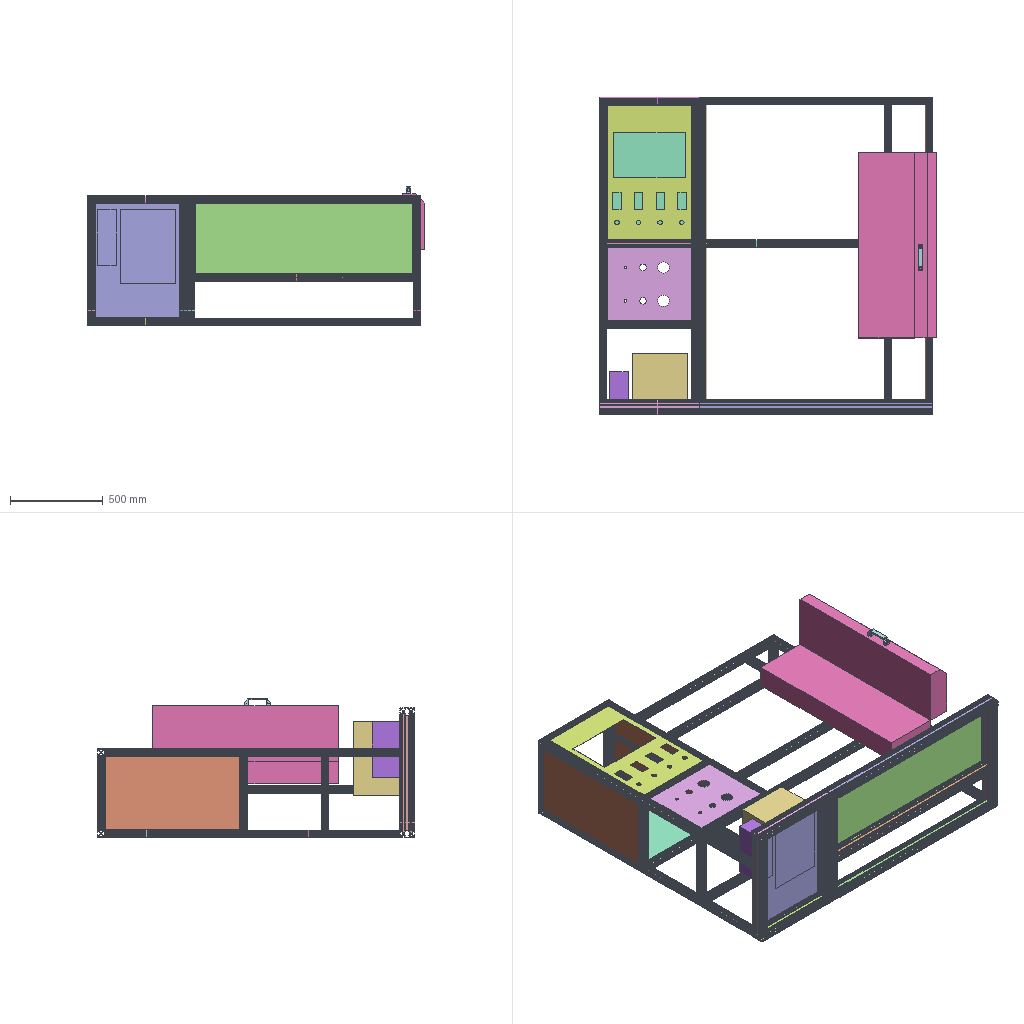Assembly | SolidWorks | 17 different items | 19 placed | box 1821 x 1715 x 750 mm
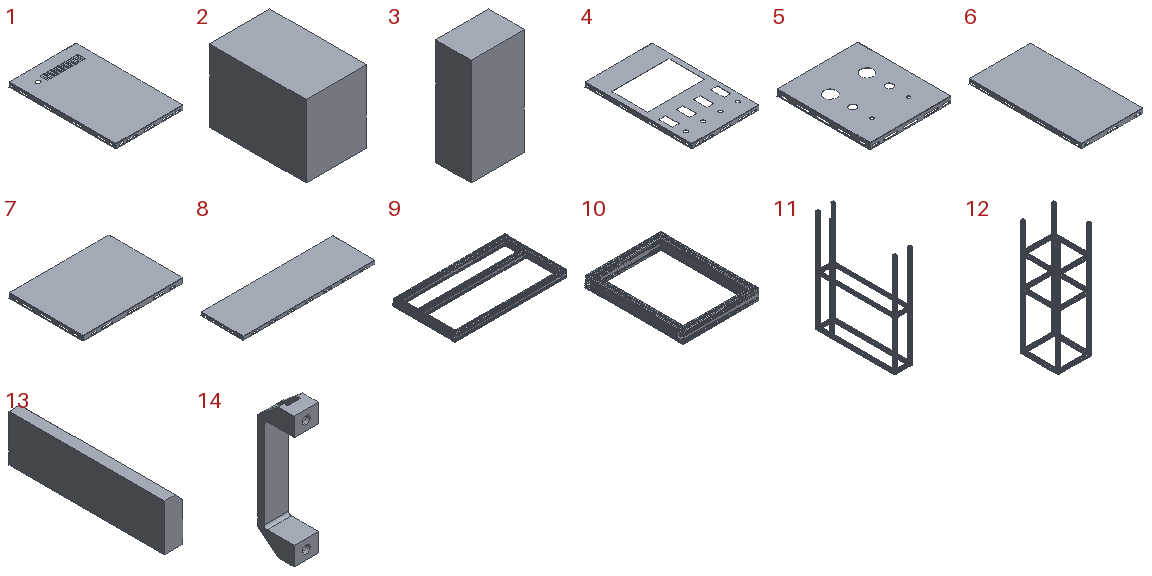Parts list (item | name | quantity | size | volume | features):
1 | - | x1 | 459 x 729 x 30 mm | 574629 mm3 | features ICE 3, EdgeFlange 1, FlatPattern 1, SMBaseFlange 1, SheetMetal 1
2 | - | x1 | 250 x 400 x 300 mm | 30000000 mm3 | features Extrusion 1
3 | - | x1 | 150 x 100 x 300 mm | 4500000 mm3 | features Extrusion 1
4 | - | x1 | 459 x 729 x 30 mm | 412274 mm3 | features ICE 3, EdgeFlange 1, FlatPattern 1, SMBaseFlange 1, SheetMetal 1
5 | - | x1 | 399 x 459 x 30 mm | 317293 mm3 | features ICE 2, Cut 1, EdgeFlange 1, FlatPattern 1, SMBaseFlange 1, SheetMetal 1
6 | - | x2 | 399 x 729 x 30 mm | 516047 mm3 | features ICE 2, EdgeFlange 1, FlatPattern 1, SMBaseFlange 1, SheetMetal 1
7 | - | x1 | 619 x 459 x 30 mm | 499692 mm3 | features ICE 2, EdgeFlange 1, FlatPattern 1, SMBaseFlange 1, SheetMetal 1
8 | - | x1 | 1179 x 379 x 30 mm | 777868 mm3 | features ICE 2, EdgeFlange 1, FlatPattern 1, SMBaseFlange 1, SheetMetal 1
9 | - | x1 | 1260 x 700.002 x 80 mm | 4888550 mm3 | features 3DProfileFeature 1, ICE 1, WeldCornerFeat 1, WeldMemberFeat 1, WeldmentFeature 1
10 | - | x1 | 540.002 x 700.002 x 80 mm | 2304321 mm3 | features 3DProfileFeature 1, ICE 1, WeldCornerFeat 1, WeldMemberFeat 1, WeldmentFeature 1
11 | - | x1 | 280 x 1260 x 1635 mm | 6460308 mm3 | features WeldCornerFeat 18, WeldMemberFeat 9, 3DProfileFeature 2, ICE 1, WeldmentFeature 1
12 | - | x1 | 480 x 540 x 1635 mm | 5554976 mm3 | features WeldCornerFeat 16, WeldMemberFeat 8, 3DProfileFeature 1, ICE 1, WeldmentFeature 1
13 | - | x2 | 120 x 1000 x 300 mm | 34750000 mm3 | features Chamfer 1, Extrusion 1
14 | - | x1 | 26 x 39 x 140 mm | 37768 mm3 | features BaseBody 1
15 | E-DEPN-W1-80-N(JLC FA) | x1 | - | - | -
16 | Base Plate2 | x1 | - | - | -
17 | Base Plate5 | x1 | - | - | -
Mates (type | each side: item.copy, entity, surface, feature):
Coincident | 10.1 plane | assembly plane | 3 times
Coincident | 12.1 face plane Aluminum Profile 40 X 40L X R4.5(6) | 4.1 face plane Base-Flange1
Width | 4.1 face plane Edge-Flange1 | 4.1 face plane Edge-Flange1 | 12.1 face plane Aluminum Profile 40 X 40L X R4.5(1) | 12.1 face plane Aluminum Profile 40 X 40L X R4.5(1)
Width | 4.1 face plane Edge-Flange1 | 4.1 face plane Edge-Flange1 | 12.1 face plane Aluminum Profile 40 X 40L X R4.5(6) | 12.1 face plane Aluminum Profile 40 X 40L X R4.5(2)
Width | 6.1 face plane Edge-Flange1 | 6.1 face plane Edge-Flange1 | 12.1 face plane Aluminum Profile 40 X 40L X R4.5(1) | 12.1 face plane Aluminum Profile 40 X 40L X R4.5(1)
Width | 6.1 face plane Edge-Flange1 | 6.1 face plane Edge-Flange1 | 12.1 face plane Aluminum Profile 40 X 40L X R4.5(2) | 12.1 face plane Aluminum Profile 40 X 40L X R4.5(10)
Coincident | 12.1 face plane Aluminum Profile 40 X 40L X R4.5(10) | 6.1 face plane Base-Flange1
Width | 1.1 face plane Edge-Flange1 | 1.1 face plane Edge-Flange1 | 12.1 face plane Aluminum Profile 40 X 40L X R4.5(6) | 12.1 face plane Aluminum Profile 40 X 40L X R4.5(2)
Width | 1.1 face plane Edge-Flange1 | 1.1 face plane Edge-Flange1 | 12.1 face plane Aluminum Profile 40 X 40L X R4.5(1) | 12.1 face plane Aluminum Profile 40 X 40L X R4.5(1)
Coincident | 12.1 face plane Aluminum Profile 40 X 40L X R4.5(2) | 1.1 face plane Base-Flange1
DistanceDim | 5.1 face plane Edge-Flange1 | 12.1 face plane Aluminum Profile 40 X 40L X R4.5(2)
Coincident | 12.1 face plane Aluminum Profile 40 X 40L X R4.5(1) | 5.1 face plane Base-Flange1
DistanceDim | 5.1 face plane Edge-Flange1 | 12.1 face plane Aluminum Profile 40 X 40L X R4.5(1)
Coincident | 13.1 face plane Boss-Extrude1 | 14.1 face plane Input1
Parallel | 13.1 face plane Boss-Extrude1 | 14.1 face plane Input1
Coincident | 13.1 edge | 13.2 edge
Coincident | 13.1 face plane Boss-Extrude1 | 13.2 face plane Boss-Extrude1
Parallel | 13.1 face plane Boss-Extrude1 | 13.2 face plane Boss-Extrude1
Coincident | 7.1 face plane Base-Flange1 | 2.1 face plane Boss-Extrude1
Coincident | 2.1 face plane Boss-Extrude1 | 3.1 face plane Boss-Extrude1 | 2 times
Coincident | 7.1 face plane Base-Flange1 | 3.1 face plane Boss-Extrude1
Coincident | 10.1 face plane Aluminum Profile 40 X 80W X R4.5(1) | 12.1 face plane Aluminum Profile 40 X 40L X R4.5(1) | 3 times
Coincident | 10.1 face plane Aluminum Profile 40 X 80W X R4.5(1) | 7.1 face plane Base-Flange1
DistanceDim | 7.1 face plane Edge-Flange1 | 10.1 face plane Aluminum Profile 40 X 80W X R4.5(1) | 2 times
Parallel | 10.1 face plane Aluminum Profile 40 X 80W X R4.5(1) | 2.1 face plane Boss-Extrude1
Coincident | 12.1 face plane Aluminum Profile 40 X 40L X R4.5(10) | 6.2 face plane Base-Flange1
DistanceDim | 6.2 face plane Edge-Flange1 | 12.1 face plane Aluminum Profile 40 X 40L X R4.5(1)
DistanceDim | 6.2 face plane Edge-Flange1 | 12.1 face plane Aluminum Profile 40 X 40L X R4.5(10)
Coincident | 10.1 face plane Aluminum Profile 40 X 80W X R4.5(1) | 9.1 face plane Aluminum Profile 40 X 80W X R4.5(1) | 4 times
Coincident | 9.1 face plane Aluminum Profile 40 X 80W X R4.5(1) | 11.1 face plane Aluminum Profile 40 X 40L X R4.5(1) | 3 times
Coincident | 8.1 face plane Base-Flange1 | 9.1 face plane Aluminum Profile 40 X 80W X R4.5(1)
DistanceDim | 8.1 face plane Edge-Flange1 | 9.1 face plane Aluminum Profile 40 X 80W X R4.5(1) | 2 times
Parallel | 13.1 face plane Boss-Extrude1 | 11.1 face plane Aluminum Profile 40 X 40L X R4.5(1)
DistanceDim | 14.1 face plane Input1 | 13.1 face plane Boss-Extrude1